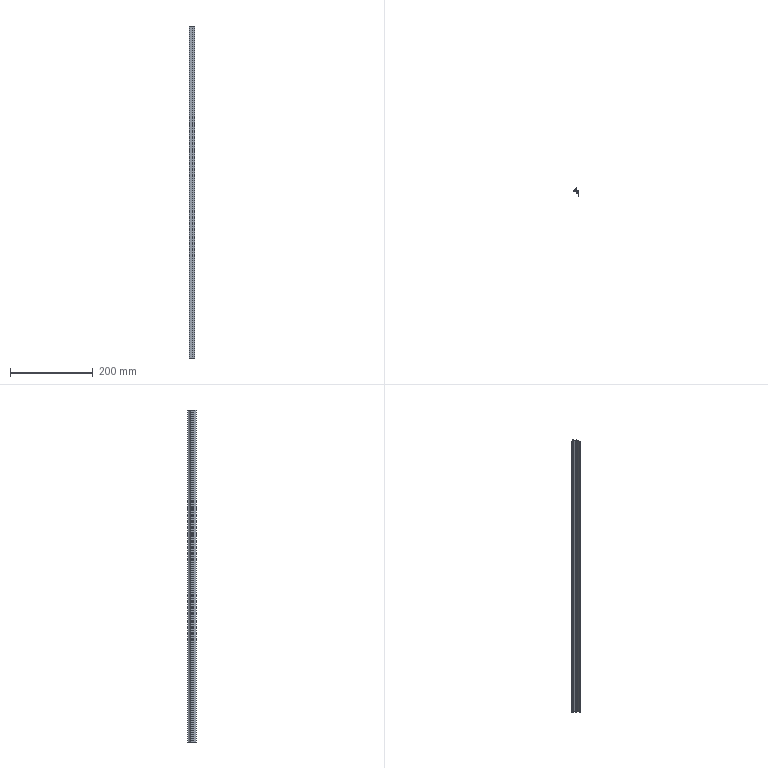Part | SolidWorks | features BaseBody 1, ICE 1, MoveFace 1 | 1 solid | 27 faces | box 14 x 20.3 x 800 mm | volume 40733 mm3 | plane 20 | cylinder 7 | commonest cylinder face diameters 0.387 x2 0.8 x2 0.4 x1 20 x1 22 x1
STEP:
#1=CARTESIAN_POINT('',(-5.304,-0.625,200.));
#2=VERTEX_POINT('',#1);
#3=CARTESIAN_POINT('',(-5.449,-0.8125,200.));
#4=VERTEX_POINT('',#3);
#5=CARTESIAN_POINT('',(-5.255,-0.8125,200.));
#6=DIRECTION('',(0.,0.,1.));
#7=DIRECTION('',(-1.,0.,0.));
#8=AXIS2_PLACEMENT_3D('',#5,#6,#7);
#9=CIRCLE('',#8,0.1937);
#10=EDGE_CURVE('',#2,#4,#9,.T.);
#11=ORIENTED_EDGE('',*,*,#10,.T.);
#12=CARTESIAN_POINT('',(-5.449,-0.8125,-600.));
#13=VERTEX_POINT('',#12);
#14=CARTESIAN_POINT('',(-5.449,-0.8125,230.));
#15=DIRECTION('',(0.,0.,-1.));
#16=VECTOR('',#15,1000.);
#17=LINE('',#14,#16);
#18=EDGE_CURVE('',#4,#13,#17,.T.);
#19=ORIENTED_EDGE('',*,*,#18,.T.);
#20=CARTESIAN_POINT('',(-5.304,-0.625,-600.));
#21=VERTEX_POINT('',#20);
#22=CARTESIAN_POINT('',(-5.255,-0.8125,-600.));
#23=DIRECTION('',(0.,0.,-1.));
#24=DIRECTION('',(1.,0.,0.));
#25=AXIS2_PLACEMENT_3D('',#22,#23,#24);
#26=CIRCLE('',#25,0.1937);
#27=EDGE_CURVE('',#13,#21,#26,.T.);
#28=ORIENTED_EDGE('',*,*,#27,.T.);
#29=CARTESIAN_POINT('',(-5.304,-0.625,230.));
#30=DIRECTION('',(0.,0.,-1.));
#31=VECTOR('',#30,1000.);
#32=LINE('',#29,#31);
#33=EDGE_CURVE('',#2,#21,#32,.T.);
#34=ORIENTED_EDGE('',*,*,#33,.F.);
#35=EDGE_LOOP('',(#11,#19,#28,#34));
#36=FACE_OUTER_BOUND('',#35,.T.);
#37=CARTESIAN_POINT('',(-5.255,-0.8125,230.));
#38=DIRECTION('',(0.,0.,-1.));
#39=DIRECTION('',(-1.,0.,0.));
#40=AXIS2_PLACEMENT_3D('',#37,#38,#39);
#41=CYLINDRICAL_SURFACE('',#40,0.1937);
#42=ADVANCED_FACE('',(#36),#41,.F.);
#43=CARTESIAN_POINT('',(5.,-1.,-600.));
#44=VERTEX_POINT('',#43);
#45=CARTESIAN_POINT('',(5.,-14.3,-600.));
#46=VERTEX_POINT('',#45);
#47=CARTESIAN_POINT('',(5.,29.623,-600.));
#48=DIRECTION('',(0.,-1.,0.));
#49=VECTOR('',#48,1000.);
#50=LINE('',#47,#49);
#51=EDGE_CURVE('',#44,#46,#50,.T.);
#52=ORIENTED_EDGE('',*,*,#51,.F.);
#53=CARTESIAN_POINT('',(5.,-1.,200.));
#54=VERTEX_POINT('',#53);
#55=CARTESIAN_POINT('',(5.,-1.,230.));
#56=DIRECTION('',(0.,0.,-1.));
#57=VECTOR('',#56,1000.);
#58=LINE('',#55,#57);
#59=EDGE_CURVE('',#54,#44,#58,.T.);
#60=ORIENTED_EDGE('',*,*,#59,.F.);
#61=CARTESIAN_POINT('',(5.,-14.3,200.));
#62=VERTEX_POINT('',#61);
#63=CARTESIAN_POINT('',(5.,-14.3,200.));
#64=DIRECTION('',(0.,1.,0.));
#65=VECTOR('',#64,1000.);
#66=LINE('',#63,#65);
#67=EDGE_CURVE('',#62,#54,#66,.T.);
#68=ORIENTED_EDGE('',*,*,#67,.F.);
#69=CARTESIAN_POINT('',(5.,-14.3,230.));
#70=DIRECTION('',(0.,0.,1.));
#71=VECTOR('',#70,1000.);
#72=LINE('',#69,#71);
#73=EDGE_CURVE('',#46,#62,#72,.T.);
#74=ORIENTED_EDGE('',*,*,#73,.F.);
#75=EDGE_LOOP('',(#52,#60,#68,#74));
#76=FACE_OUTER_BOUND('',#75,.T.);
#77=CARTESIAN_POINT('',(5.,-14.3,230.));
#78=DIRECTION('',(-1.,0.,0.));
#79=DIRECTION('',(0.,0.,1.));
#80=AXIS2_PLACEMENT_3D('',#77,#78,#79);
#81=PLANE('',#80);
#82=ADVANCED_FACE('',(#76),#81,.F.);
#83=CARTESIAN_POINT('',(-9.,-2.,-600.));
#84=VERTEX_POINT('',#83);
#85=CARTESIAN_POINT('',(-9.,-2.,200.));
#86=VERTEX_POINT('',#85);
#87=CARTESIAN_POINT('',(-9.,-2.,230.));
#88=DIRECTION('',(0.,0.,1.));
#89=VECTOR('',#88,1000.);
#90=LINE('',#87,#89);
#91=EDGE_CURVE('',#84,#86,#90,.T.);
#92=ORIENTED_EDGE('',*,*,#91,.F.);
#93=CARTESIAN_POINT('',(0.9,-2.,-600.));
#94=VERTEX_POINT('',#93);
#95=CARTESIAN_POINT('',(5.,-2.,-600.));
#96=DIRECTION('',(-1.,0.,0.));
#97=VECTOR('',#96,1000.);
#98=LINE('',#95,#97);
#99=EDGE_CURVE('',#94,#84,#98,.T.);
#100=ORIENTED_EDGE('',*,*,#99,.F.);
#101=CARTESIAN_POINT('',(0.9,-2.,200.));
#102=VERTEX_POINT('',#101);
#103=CARTESIAN_POINT('',(0.9,-2.,230.));
#104=DIRECTION('',(0.,0.,-1.));
#105=VECTOR('',#104,1000.);
#106=LINE('',#103,#105);
#107=EDGE_CURVE('',#102,#94,#106,.T.);
#108=ORIENTED_EDGE('',*,*,#107,.F.);
#109=CARTESIAN_POINT('',(5.,-2.,200.));
#110=DIRECTION('',(1.,0.,0.));
#111=VECTOR('',#110,1000.);
#112=LINE('',#109,#111);
#113=EDGE_CURVE('',#86,#102,#112,.T.);
#114=ORIENTED_EDGE('',*,*,#113,.F.);
#115=EDGE_LOOP('',(#92,#100,#108,#114));
#116=FACE_OUTER_BOUND('',#115,.T.);
#117=CARTESIAN_POINT('',(-9.,-2.,230.));
#118=DIRECTION('',(0.,1.,0.));
#119=DIRECTION('',(0.,0.,1.));
#120=AXIS2_PLACEMENT_3D('',#117,#118,#119);
#121=PLANE('',#120);
#122=ADVANCED_FACE('',(#116),#121,.F.);
#123=CARTESIAN_POINT('',(4.,-6.,200.));
#124=VERTEX_POINT('',#123);
#125=CARTESIAN_POINT('',(4.,-3.,200.));
#126=VERTEX_POINT('',#125);
#127=CARTESIAN_POINT('',(4.,29.623,200.));
#128=DIRECTION('',(0.,1.,0.));
#129=VECTOR('',#128,1000.);
#130=LINE('',#127,#129);
#131=EDGE_CURVE('',#124,#126,#130,.T.);
#132=ORIENTED_EDGE('',*,*,#131,.F.);
#133=CARTESIAN_POINT('',(1.,-6.,200.));
#134=VERTEX_POINT('',#133);
#135=CARTESIAN_POINT('',(5.,-6.,200.));
#136=DIRECTION('',(1.,0.,0.));
#137=VECTOR('',#136,1000.);
#138=LINE('',#135,#137);
#139=EDGE_CURVE('',#134,#124,#138,.T.);
#140=ORIENTED_EDGE('',*,*,#139,.F.);
#141=CARTESIAN_POINT('',(1.,-6.7,200.));
#142=VERTEX_POINT('',#141);
#143=CARTESIAN_POINT('',(1.,-6.,200.));
#144=DIRECTION('',(0.,-1.,0.));
#145=VECTOR('',#144,1000.);
#146=LINE('',#143,#145);
#147=EDGE_CURVE('',#134,#142,#146,.T.);
#148=ORIENTED_EDGE('',*,*,#147,.T.);
#149=CARTESIAN_POINT('',(-1.7,-6.7,200.));
#150=VERTEX_POINT('',#149);
#151=CARTESIAN_POINT('',(5.,-6.7,200.));
#152=DIRECTION('',(1.,0.,0.));
#153=VECTOR('',#152,1000.);
#154=LINE('',#151,#153);
#155=EDGE_CURVE('',#150,#142,#154,.T.);
#156=ORIENTED_EDGE('',*,*,#155,.F.);
#157=CARTESIAN_POINT('',(-1.7,-7.7,200.));
#158=VERTEX_POINT('',#157);
#159=CARTESIAN_POINT('',(-1.7,-6.7,200.));
#160=DIRECTION('',(0.,-1.,0.));
#161=VECTOR('',#160,1000.);
#162=LINE('',#159,#161);
#163=EDGE_CURVE('',#150,#158,#162,.T.);
#164=ORIENTED_EDGE('',*,*,#163,.T.);
#165=CARTESIAN_POINT('',(4.,-7.7,200.));
#166=VERTEX_POINT('',#165);
#167=CARTESIAN_POINT('',(5.,-7.7,200.));
#168=DIRECTION('',(-1.,0.,0.));
#169=VECTOR('',#168,1000.);
#170=LINE('',#167,#169);
#171=EDGE_CURVE('',#166,#158,#170,.T.);
#172=ORIENTED_EDGE('',*,*,#171,.F.);
#173=CARTESIAN_POINT('',(4.,-14.3,200.));
#174=VERTEX_POINT('',#173);
#175=CARTESIAN_POINT('',(4.,29.623,200.));
#176=DIRECTION('',(0.,1.,0.));
#177=VECTOR('',#176,1000.);
#178=LINE('',#175,#177);
#179=EDGE_CURVE('',#174,#166,#178,.T.);
#180=ORIENTED_EDGE('',*,*,#179,.F.);
#181=CARTESIAN_POINT('',(5.,-14.3,200.));
#182=DIRECTION('',(-1.,0.,0.));
#183=VECTOR('',#182,1000.);
#184=LINE('',#181,#183);
#185=EDGE_CURVE('',#62,#174,#184,.T.);
#186=ORIENTED_EDGE('',*,*,#185,.F.);
#187=ORIENTED_EDGE('',*,*,#67,.T.);
#188=CARTESIAN_POINT('',(-5.207,-1.,200.));
#189=VERTEX_POINT('',#188);
#190=CARTESIAN_POINT('',(5.,-1.,200.));
#191=DIRECTION('',(1.,0.,0.));
#192=VECTOR('',#191,1000.);
#193=LINE('',#190,#192);
#194=EDGE_CURVE('',#189,#54,#193,.T.);
#195=ORIENTED_EDGE('',*,*,#194,.F.);
#196=CARTESIAN_POINT('',(-5.255,-0.8125,200.));
#197=DIRECTION('',(0.,0.,1.));
#198=DIRECTION('',(-1.,0.,0.));
#199=AXIS2_PLACEMENT_3D('',#196,#197,#198);
#200=CIRCLE('',#199,0.1937);
#201=EDGE_CURVE('',#4,#189,#200,.T.);
#202=ORIENTED_EDGE('',*,*,#201,.F.);
#203=ORIENTED_EDGE('',*,*,#10,.F.);
#204=CARTESIAN_POINT('',(-1.368,3.063,200.));
#205=VERTEX_POINT('',#204);
#206=CARTESIAN_POINT('',(-10.628,9.,200.));
#207=DIRECTION('',(0.,0.,1.));
#208=DIRECTION('',(-1.,0.,0.));
#209=AXIS2_PLACEMENT_3D('',#206,#207,#208);
#210=CIRCLE('',#209,11.);
#211=EDGE_CURVE('',#2,#205,#210,.T.);
#212=ORIENTED_EDGE('',*,*,#211,.T.);
#213=CARTESIAN_POINT('',(-1.,2.955,200.));
#214=VERTEX_POINT('',#213);
#215=CARTESIAN_POINT('',(-1.2,2.955,200.));
#216=DIRECTION('',(0.,0.,1.));
#217=DIRECTION('',(-1.,0.,0.));
#218=AXIS2_PLACEMENT_3D('',#215,#216,#217);
#219=CIRCLE('',#218,0.2);
#220=EDGE_CURVE('',#214,#205,#219,.T.);
#221=ORIENTED_EDGE('',*,*,#220,.F.);
#222=CARTESIAN_POINT('',(-1.,1.5,200.));
#223=VERTEX_POINT('',#222);
#224=CARTESIAN_POINT('',(-1.,2.955,200.));
#225=DIRECTION('',(0.,1.,0.));
#226=VECTOR('',#225,1000.);
#227=LINE('',#224,#226);
#228=EDGE_CURVE('',#223,#214,#227,.T.);
#229=ORIENTED_EDGE('',*,*,#228,.F.);
#230=CARTESIAN_POINT('',(0.,1.5,200.));
#231=VERTEX_POINT('',#230);
#232=CARTESIAN_POINT('',(-1.,1.5,200.));
#233=DIRECTION('',(-1.,0.,0.));
#234=VECTOR('',#233,1000.);
#235=LINE('',#232,#234);
#236=EDGE_CURVE('',#231,#223,#235,.T.);
#237=ORIENTED_EDGE('',*,*,#236,.F.);
#238=CARTESIAN_POINT('',(0.,6.,200.));
#239=VERTEX_POINT('',#238);
#240=CARTESIAN_POINT('',(0.,1.5,200.));
#241=DIRECTION('',(0.,-1.,0.));
#242=VECTOR('',#241,1000.);
#243=LINE('',#240,#242);
#244=EDGE_CURVE('',#239,#231,#243,.T.);
#245=ORIENTED_EDGE('',*,*,#244,.F.);
#246=CARTESIAN_POINT('',(-0.8,6.,200.));
#247=VERTEX_POINT('',#246);
#248=CARTESIAN_POINT('',(0.,6.,200.));
#249=DIRECTION('',(1.,0.,0.));
#250=VECTOR('',#249,1000.);
#251=LINE('',#248,#250);
#252=EDGE_CURVE('',#247,#239,#251,.T.);
#253=ORIENTED_EDGE('',*,*,#252,.F.);
#254=CARTESIAN_POINT('',(-1.178,5.731,200.));
#255=VERTEX_POINT('',#254);
#256=CARTESIAN_POINT('',(-0.8,5.6,200.));
#257=DIRECTION('',(0.,0.,1.));
#258=DIRECTION('',(-1.,0.,0.));
#259=AXIS2_PLACEMENT_3D('',#256,#257,#258);
#260=CIRCLE('',#259,0.4);
#261=EDGE_CURVE('',#247,#255,#260,.T.);
#262=ORIENTED_EDGE('',*,*,#261,.T.);
#263=CARTESIAN_POINT('',(-8.678,-0.8077,200.));
#264=VERTEX_POINT('',#263);
#265=CARTESIAN_POINT('',(-10.628,9.,200.));
#266=DIRECTION('',(0.,0.,1.));
#267=DIRECTION('',(-1.,0.,0.));
#268=AXIS2_PLACEMENT_3D('',#265,#266,#267);
#269=CIRCLE('',#268,10.);
#270=EDGE_CURVE('',#264,#255,#269,.T.);
#271=ORIENTED_EDGE('',*,*,#270,.F.);
#272=CARTESIAN_POINT('',(-9.,-1.2,200.));
#273=VERTEX_POINT('',#272);
#274=CARTESIAN_POINT('',(-8.6,-1.2,200.));
#275=DIRECTION('',(0.,0.,1.));
#276=DIRECTION('',(-1.,0.,0.));
#277=AXIS2_PLACEMENT_3D('',#274,#275,#276);
#278=CIRCLE('',#277,0.4);
#279=EDGE_CURVE('',#264,#273,#278,.T.);
#280=ORIENTED_EDGE('',*,*,#279,.T.);
#281=CARTESIAN_POINT('',(-9.,8.,200.));
#282=DIRECTION('',(0.,-1.,0.));
#283=VECTOR('',#282,1000.);
#284=LINE('',#281,#283);
#285=EDGE_CURVE('',#273,#86,#284,.T.);
#286=ORIENTED_EDGE('',*,*,#285,.T.);
#287=ORIENTED_EDGE('',*,*,#113,.T.);
#288=CARTESIAN_POINT('',(0.9,-3.,200.));
#289=VERTEX_POINT('',#288);
#290=CARTESIAN_POINT('',(0.9,29.623,200.));
#291=DIRECTION('',(0.,1.,0.));
#292=VECTOR('',#291,1000.);
#293=LINE('',#290,#292);
#294=EDGE_CURVE('',#289,#102,#293,.T.);
#295=ORIENTED_EDGE('',*,*,#294,.F.);
#296=CARTESIAN_POINT('',(5.,-3.,200.));
#297=DIRECTION('',(-1.,0.,0.));
#298=VECTOR('',#297,1000.);
#299=LINE('',#296,#298);
#300=EDGE_CURVE('',#126,#289,#299,.T.);
#301=ORIENTED_EDGE('',*,*,#300,.F.);
#302=EDGE_LOOP('',(#132,#140,#148,#156,#164,#172,#180,#186,#187,#195,#202,#203,#212,#221,#229,#237,#245,#253,#262,#271,#280,#286,#287,#295,#301));
#303=FACE_OUTER_BOUND('',#302,.T.);
#304=CARTESIAN_POINT('',(5.,29.623,200.));
#305=DIRECTION('',(0.,0.,-1.));
#306=DIRECTION('',(-1.,0.,0.));
#307=AXIS2_PLACEMENT_3D('',#304,#305,#306);
#308=PLANE('',#307);
#309=ADVANCED_FACE('',(#303),#308,.F.);
#310=ORIENTED_EDGE('',*,*,#185,.T.);
#311=CARTESIAN_POINT('',(4.,-14.3,-600.));
#312=VERTEX_POINT('',#311);
#313=CARTESIAN_POINT('',(4.,-14.3,230.));
#314=DIRECTION('',(0.,0.,1.));
#315=VECTOR('',#314,1000.);
#316=LINE('',#313,#315);
#317=EDGE_CURVE('',#312,#174,#316,.T.);
#318=ORIENTED_EDGE('',*,*,#317,.F.);
#319=CARTESIAN_POINT('',(5.,-14.3,-600.));
#320=DIRECTION('',(-1.,0.,0.));
#321=VECTOR('',#320,1000.);
#322=LINE('',#319,#321);
#323=EDGE_CURVE('',#46,#312,#322,.T.);
#324=ORIENTED_EDGE('',*,*,#323,.F.);
#325=ORIENTED_EDGE('',*,*,#73,.T.);
#326=EDGE_LOOP('',(#310,#318,#324,#325));
#327=FACE_OUTER_BOUND('',#326,.T.);
#328=CARTESIAN_POINT('',(4.,-14.3,230.));
#329=DIRECTION('',(0.,1.,0.));
#330=DIRECTION('',(0.,0.,1.));
#331=AXIS2_PLACEMENT_3D('',#328,#329,#330);
#332=PLANE('',#331);
#333=ADVANCED_FACE('',(#327),#332,.F.);
#334=ORIENTED_EDGE('',*,*,#51,.T.);
#335=ORIENTED_EDGE('',*,*,#323,.T.);
#336=CARTESIAN_POINT('',(4.,-7.7,-600.));
#337=VERTEX_POINT('',#336);
#338=CARTESIAN_POINT('',(4.,-7.7,-600.));
#339=DIRECTION('',(0.,-1.,0.));
#340=VECTOR('',#339,1000.);
#341=LINE('',#338,#340);
#342=EDGE_CURVE('',#337,#312,#341,.T.);
#343=ORIENTED_EDGE('',*,*,#342,.F.);
#344=CARTESIAN_POINT('',(-1.7,-7.7,-600.));
#345=VERTEX_POINT('',#344);
#346=CARTESIAN_POINT('',(-1.7,-7.7,-600.));
#347=DIRECTION('',(1.,0.,0.));
#348=VECTOR('',#347,1000.);
#349=LINE('',#346,#348);
#350=EDGE_CURVE('',#345,#337,#349,.T.);
#351=ORIENTED_EDGE('',*,*,#350,.F.);
#352=CARTESIAN_POINT('',(-1.7,-6.7,-600.));
#353=VERTEX_POINT('',#352);
#354=CARTESIAN_POINT('',(-1.7,29.623,-600.));
#355=DIRECTION('',(0.,1.,0.));
#356=VECTOR('',#355,1000.);
#357=LINE('',#354,#356);
#358=EDGE_CURVE('',#345,#353,#357,.T.);
#359=ORIENTED_EDGE('',*,*,#358,.T.);
#360=CARTESIAN_POINT('',(1.,-6.7,-600.));
#361=VERTEX_POINT('',#360);
#362=CARTESIAN_POINT('',(1.,-6.7,-600.));
#363=DIRECTION('',(-1.,0.,0.));
#364=VECTOR('',#363,1000.);
#365=LINE('',#362,#364);
#366=EDGE_CURVE('',#361,#353,#365,.T.);
#367=ORIENTED_EDGE('',*,*,#366,.F.);
#368=CARTESIAN_POINT('',(1.,-6.,-600.));
#369=VERTEX_POINT('',#368);
#370=CARTESIAN_POINT('',(1.,29.623,-600.));
#371=DIRECTION('',(0.,1.,0.));
#372=VECTOR('',#371,1000.);
#373=LINE('',#370,#372);
#374=EDGE_CURVE('',#361,#369,#373,.T.);
#375=ORIENTED_EDGE('',*,*,#374,.T.);
#376=CARTESIAN_POINT('',(4.,-6.,-600.));
#377=VERTEX_POINT('',#376);
#378=CARTESIAN_POINT('',(4.,-6.,-600.));
#379=DIRECTION('',(-1.,0.,0.));
#380=VECTOR('',#379,1000.);
#381=LINE('',#378,#380);
#382=EDGE_CURVE('',#377,#369,#381,.T.);
#383=ORIENTED_EDGE('',*,*,#382,.F.);
#384=CARTESIAN_POINT('',(4.,-3.,-600.));
#385=VERTEX_POINT('',#384);
#386=CARTESIAN_POINT('',(4.,-3.,-600.));
#387=DIRECTION('',(0.,-1.,0.));
#388=VECTOR('',#387,1000.);
#389=LINE('',#386,#388);
#390=EDGE_CURVE('',#385,#377,#389,.T.);
#391=ORIENTED_EDGE('',*,*,#390,.F.);
#392=CARTESIAN_POINT('',(0.9,-3.,-600.));
#393=VERTEX_POINT('',#392);
#394=CARTESIAN_POINT('',(0.9,-3.,-600.));
#395=DIRECTION('',(1.,0.,0.));
#396=VECTOR('',#395,1000.);
#397=LINE('',#394,#396);
#398=EDGE_CURVE('',#393,#385,#397,.T.);
#399=ORIENTED_EDGE('',*,*,#398,.F.);
#400=CARTESIAN_POINT('',(0.9,-2.,-600.));
#401=DIRECTION('',(0.,-1.,0.));
#402=VECTOR('',#401,1000.);
#403=LINE('',#400,#402);
#404=EDGE_CURVE('',#94,#393,#403,.T.);
#405=ORIENTED_EDGE('',*,*,#404,.F.);
#406=ORIENTED_EDGE('',*,*,#99,.T.);
#407=CARTESIAN_POINT('',(-9.,-1.2,-600.));
#408=VERTEX_POINT('',#407);
#409=CARTESIAN_POINT('',(-9.,-1.2,-600.));
#410=DIRECTION('',(0.,-1.,0.));
#411=VECTOR('',#410,1000.);
#412=LINE('',#409,#411);
#413=EDGE_CURVE('',#408,#84,#412,.T.);
#414=ORIENTED_EDGE('',*,*,#413,.F.);
#415=CARTESIAN_POINT('',(-8.678,-0.8077,-600.));
#416=VERTEX_POINT('',#415);
#417=CARTESIAN_POINT('',(-8.6,-1.2,-600.));
#418=DIRECTION('',(0.,0.,-1.));
#419=DIRECTION('',(1.,0.,0.));
#420=AXIS2_PLACEMENT_3D('',#417,#418,#419);
#421=CIRCLE('',#420,0.4);
#422=EDGE_CURVE('',#408,#416,#421,.T.);
#423=ORIENTED_EDGE('',*,*,#422,.T.);
#424=CARTESIAN_POINT('',(-1.178,5.731,-600.));
#425=VERTEX_POINT('',#424);
#426=CARTESIAN_POINT('',(-10.628,9.,-600.));
#427=DIRECTION('',(0.,0.,-1.));
#428=DIRECTION('',(1.,0.,0.));
#429=AXIS2_PLACEMENT_3D('',#426,#427,#428);
#430=CIRCLE('',#429,10.);
#431=EDGE_CURVE('',#425,#416,#430,.T.);
#432=ORIENTED_EDGE('',*,*,#431,.F.);
#433=CARTESIAN_POINT('',(-0.8,6.,-600.));
#434=VERTEX_POINT('',#433);
#435=CARTESIAN_POINT('',(-0.8,5.6,-600.));
#436=DIRECTION('',(0.,0.,-1.));
#437=DIRECTION('',(1.,0.,0.));
#438=AXIS2_PLACEMENT_3D('',#435,#436,#437);
#439=CIRCLE('',#438,0.4);
#440=EDGE_CURVE('',#425,#434,#439,.T.);
#441=ORIENTED_EDGE('',*,*,#440,.T.);
#442=CARTESIAN_POINT('',(0.,6.,-600.));
#443=VERTEX_POINT('',#442);
#444=CARTESIAN_POINT('',(0.,6.,-600.));
#445=DIRECTION('',(-1.,0.,0.));
#446=VECTOR('',#445,1000.);
#447=LINE('',#444,#446);
#448=EDGE_CURVE('',#443,#434,#447,.T.);
#449=ORIENTED_EDGE('',*,*,#448,.F.);
#450=CARTESIAN_POINT('',(0.,1.5,-600.));
#451=VERTEX_POINT('',#450);
#452=CARTESIAN_POINT('',(0.,1.5,-600.));
#453=DIRECTION('',(0.,1.,0.));
#454=VECTOR('',#453,1000.);
#455=LINE('',#452,#454);
#456=EDGE_CURVE('',#451,#443,#455,.T.);
#457=ORIENTED_EDGE('',*,*,#456,.F.);
#458=CARTESIAN_POINT('',(-1.,1.5,-600.));
#459=VERTEX_POINT('',#458);
#460=CARTESIAN_POINT('',(-1.,1.5,-600.));
#461=DIRECTION('',(1.,0.,0.));
#462=VECTOR('',#461,1000.);
#463=LINE('',#460,#462);
#464=EDGE_CURVE('',#459,#451,#463,.T.);
#465=ORIENTED_EDGE('',*,*,#464,.F.);
#466=CARTESIAN_POINT('',(-1.,2.955,-600.));
#467=VERTEX_POINT('',#466);
#468=CARTESIAN_POINT('',(-1.,2.955,-600.));
#469=DIRECTION('',(0.,-1.,0.));
#470=VECTOR('',#469,1000.);
#471=LINE('',#468,#470);
#472=EDGE_CURVE('',#467,#459,#471,.T.);
#473=ORIENTED_EDGE('',*,*,#472,.F.);
#474=CARTESIAN_POINT('',(-1.368,3.063,-600.));
#475=VERTEX_POINT('',#474);
#476=CARTESIAN_POINT('',(-1.2,2.955,-600.));
#477=DIRECTION('',(0.,0.,-1.));
#478=DIRECTION('',(1.,0.,0.));
#479=AXIS2_PLACEMENT_3D('',#476,#477,#478);
#480=CIRCLE('',#479,0.2);
#481=EDGE_CURVE('',#475,#467,#480,.T.);
#482=ORIENTED_EDGE('',*,*,#481,.F.);
#483=CARTESIAN_POINT('',(-10.628,9.,-600.));
#484=DIRECTION('',(0.,0.,-1.));
#485=DIRECTION('',(1.,0.,0.));
#486=AXIS2_PLACEMENT_3D('',#483,#484,#485);
#487=CIRCLE('',#486,11.);
#488=EDGE_CURVE('',#475,#21,#487,.T.);
#489=ORIENTED_EDGE('',*,*,#488,.T.);
#490=ORIENTED_EDGE('',*,*,#27,.F.);
#491=CARTESIAN_POINT('',(-5.207,-1.,-600.));
#492=VERTEX_POINT('',#491);
#493=CARTESIAN_POINT('',(-5.255,-0.8125,-600.));
#494=DIRECTION('',(0.,0.,-1.));
#495=DIRECTION('',(1.,0.,0.));
#496=AXIS2_PLACEMENT_3D('',#493,#494,#495);
#497=CIRCLE('',#496,0.1937);
#498=EDGE_CURVE('',#492,#13,#497,.T.);
#499=ORIENTED_EDGE('',*,*,#498,.F.);
#500=CARTESIAN_POINT('',(5.,-1.,-600.));
#501=DIRECTION('',(-1.,0.,0.));
#502=VECTOR('',#501,1000.);
#503=LINE('',#500,#502);
#504=EDGE_CURVE('',#44,#492,#503,.T.);
#505=ORIENTED_EDGE('',*,*,#504,.F.);
#506=EDGE_LOOP('',(#334,#335,#343,#351,#359,#367,#375,#383,#391,#399,#405,#406,#414,#423,#432,#441,#449,#457,#465,#473,#482,#489,#490,#499,#505));
#507=FACE_OUTER_BOUND('',#506,.T.);
#508=CARTESIAN_POINT('',(5.,29.623,-600.));
#509=DIRECTION('',(0.,0.,1.));
#510=DIRECTION('',(1.,0.,0.));
#511=AXIS2_PLACEMENT_3D('',#508,#509,#510);
#512=PLANE('',#511);
#513=ADVANCED_FACE('',(#507),#512,.F.);
#514=ORIENTED_EDGE('',*,*,#59,.T.);
#515=ORIENTED_EDGE('',*,*,#504,.T.);
#516=CARTESIAN_POINT('',(-5.207,-1.,230.));
#517=DIRECTION('',(0.,0.,-1.));
#518=VECTOR('',#517,1000.);
#519=LINE('',#516,#518);
#520=EDGE_CURVE('',#189,#492,#519,.T.);
#521=ORIENTED_EDGE('',*,*,#520,.F.);
#522=ORIENTED_EDGE('',*,*,#194,.T.);
#523=EDGE_LOOP('',(#514,#515,#521,#522));
#524=FACE_OUTER_BOUND('',#523,.T.);
#525=CARTESIAN_POINT('',(5.,-1.,230.));
#526=DIRECTION('',(0.,-1.,0.));
#527=DIRECTION('',(0.,0.,-1.));
#528=AXIS2_PLACEMENT_3D('',#525,#526,#527);
#529=PLANE('',#528);
#530=ADVANCED_FACE('',(#524),#529,.F.);
#531=CARTESIAN_POINT('',(-9.,-1.2,230.));
#532=DIRECTION('',(0.,0.,1.));
#533=VECTOR('',#532,1000.);
#534=LINE('',#531,#533);
#535=EDGE_CURVE('',#408,#273,#534,.T.);
#536=ORIENTED_EDGE('',*,*,#535,.F.);
#537=ORIENTED_EDGE('',*,*,#413,.T.);
#538=ORIENTED_EDGE('',*,*,#91,.T.);
#539=ORIENTED_EDGE('',*,*,#285,.F.);
#540=EDGE_LOOP('',(#536,#537,#538,#539));
#541=FACE_OUTER_BOUND('',#540,.T.);
#542=CARTESIAN_POINT('',(-9.,-1.2,230.));
#543=DIRECTION('',(1.,0.,0.));
#544=DIRECTION('',(0.,0.,-1.));
#545=AXIS2_PLACEMENT_3D('',#542,#543,#544);
#546=PLANE('',#545);
#547=ADVANCED_FACE('',(#541),#546,.F.);
#548=ORIENTED_EDGE('',*,*,#294,.T.);
#549=ORIENTED_EDGE('',*,*,#107,.T.);
#550=ORIENTED_EDGE('',*,*,#404,.T.);
#551=CARTESIAN_POINT('',(0.9,-3.,230.));
#552=DIRECTION('',(0.,0.,-1.));
#553=VECTOR('',#552,1000.);
#554=LINE('',#551,#553);
#555=EDGE_CURVE('',#289,#393,#554,.T.);
#556=ORIENTED_EDGE('',*,*,#555,.F.);
#557=EDGE_LOOP('',(#548,#549,#550,#556));
#558=FACE_OUTER_BOUND('',#557,.T.);
#559=CARTESIAN_POINT('',(0.9,-2.,230.));
#560=DIRECTION('',(1.,0.,0.));
#561=DIRECTION('',(0.,0.,-1.));
#562=AXIS2_PLACEMENT_3D('',#559,#560,#561);
#563=PLANE('',#562);
#564=ADVANCED_FACE('',(#558),#563,.F.);
#565=ORIENTED_EDGE('',*,*,#300,.T.);
#566=ORIENTED_EDGE('',*,*,#555,.T.);
#567=ORIENTED_EDGE('',*,*,#398,.T.);
#568=CARTESIAN_POINT('',(4.,-3.,230.));
#569=DIRECTION('',(0.,0.,-1.));
#570=VECTOR('',#569,1000.);
#571=LINE('',#568,#570);
#572=EDGE_CURVE('',#126,#385,#571,.T.);
#573=ORIENTED_EDGE('',*,*,#572,.F.);
#574=EDGE_LOOP('',(#565,#566,#567,#573));
#575=FACE_OUTER_BOUND('',#574,.T.);
#576=CARTESIAN_POINT('',(0.9,-3.,230.));
#577=DIRECTION('',(0.,1.,0.));
#578=DIRECTION('',(0.,0.,1.));
#579=AXIS2_PLACEMENT_3D('',#576,#577,#578);
#580=PLANE('',#579);
#581=ADVANCED_FACE('',(#575),#580,.F.);
#582=ORIENTED_EDGE('',*,*,#131,.T.);
#583=ORIENTED_EDGE('',*,*,#572,.T.);
#584=ORIENTED_EDGE('',*,*,#390,.T.);
#585=CARTESIAN_POINT('',(4.,-6.,230.));
#586=DIRECTION('',(0.,0.,-1.));
#587=VECTOR('',#586,1000.);
#588=LINE('',#585,#587);
#589=EDGE_CURVE('',#124,#377,#588,.T.);
#590=ORIENTED_EDGE('',*,*,#589,.F.);
#591=EDGE_LOOP('',(#582,#583,#584,#590));
#592=FACE_OUTER_BOUND('',#591,.T.);
#593=CARTESIAN_POINT('',(4.,-3.,230.));
#594=DIRECTION('',(1.,0.,0.));
#595=DIRECTION('',(0.,0.,-1.));
#596=AXIS2_PLACEMENT_3D('',#593,#594,#595);
#597=PLANE('',#596);
#598=ADVANCED_FACE('',(#592),#597,.F.);
#599=ORIENTED_EDGE('',*,*,#139,.T.);
#600=ORIENTED_EDGE('',*,*,#589,.T.);
#601=ORIENTED_EDGE('',*,*,#382,.T.);
#602=CARTESIAN_POINT('',(1.,-6.,230.));
#603=DIRECTION('',(0.,0.,-1.));
#604=VECTOR('',#603,1000.);
#605=LINE('',#602,#604);
#606=EDGE_CURVE('',#134,#369,#605,.T.);
#607=ORIENTED_EDGE('',*,*,#606,.F.);
#608=EDGE_LOOP('',(#599,#600,#601,#607));
#609=FACE_OUTER_BOUND('',#608,.T.);
#610=CARTESIAN_POINT('',(4.,-6.,230.));
#611=DIRECTION('',(0.,-1.,0.));
#612=DIRECTION('',(0.,0.,-1.));
#613=AXIS2_PLACEMENT_3D('',#610,#611,#612);
#614=PLANE('',#613);
#615=ADVANCED_FACE('',(#609),#614,.F.);
#616=ORIENTED_EDGE('',*,*,#155,.T.);
#617=CARTESIAN_POINT('',(1.,-6.7,230.));
#618=DIRECTION('',(0.,0.,1.));
#619=VECTOR('',#618,1000.);
#620=LINE('',#617,#619);
#621=EDGE_CURVE('',#361,#142,#620,.T.);
#622=ORIENTED_EDGE('',*,*,#621,.F.);
#623=ORIENTED_EDGE('',*,*,#366,.T.);
#624=CARTESIAN_POINT('',(-1.7,-6.7,230.));
#625=DIRECTION('',(0.,0.,-1.));
#626=VECTOR('',#625,1000.);
#627=LINE('',#624,#626);
#628=EDGE_CURVE('',#150,#353,#627,.T.);
#629=ORIENTED_EDGE('',*,*,#628,.F.);
#630=EDGE_LOOP('',(#616,#622,#623,#629));
#631=FACE_OUTER_BOUND('',#630,.T.);
#632=CARTESIAN_POINT('',(1.,-6.7,230.));
#633=DIRECTION('',(0.,-1.,0.));
#634=DIRECTION('',(0.,0.,-1.));
#635=AXIS2_PLACEMENT_3D('',#632,#633,#634);
#636=PLANE('',#635);
#637=ADVANCED_FACE('',(#631),#636,.F.);
#638=ORIENTED_EDGE('',*,*,#171,.T.);
#639=CARTESIAN_POINT('',(-1.7,-7.7,230.));
#640=DIRECTION('',(0.,0.,1.));
#641=VECTOR('',#640,1000.);
#642=LINE('',#639,#641);
#643=EDGE_CURVE('',#345,#158,#642,.T.);
#644=ORIENTED_EDGE('',*,*,#643,.F.);
#645=ORIENTED_EDGE('',*,*,#350,.T.);
#646=CARTESIAN_POINT('',(4.,-7.7,230.));
#647=DIRECTION('',(0.,0.,-1.));
#648=VECTOR('',#647,1000.);
#649=LINE('',#646,#648);
#650=EDGE_CURVE('',#166,#337,#649,.T.);
#651=ORIENTED_EDGE('',*,*,#650,.F.);
#652=EDGE_LOOP('',(#638,#644,#645,#651));
#653=FACE_OUTER_BOUND('',#652,.T.);
#654=CARTESIAN_POINT('',(-1.7,-7.7,230.));
#655=DIRECTION('',(0.,1.,0.));
#656=DIRECTION('',(0.,0.,1.));
#657=AXIS2_PLACEMENT_3D('',#654,#655,#656);
#658=PLANE('',#657);
#659=ADVANCED_FACE('',(#653),#658,.F.);
#660=ORIENTED_EDGE('',*,*,#179,.T.);
#661=ORIENTED_EDGE('',*,*,#650,.T.);
#662=ORIENTED_EDGE('',*,*,#342,.T.);
#663=ORIENTED_EDGE('',*,*,#317,.T.);
#664=EDGE_LOOP('',(#660,#661,#662,#663));
#665=FACE_OUTER_BOUND('',#664,.T.);
#666=CARTESIAN_POINT('',(4.,-7.7,230.));
#667=DIRECTION('',(1.,0.,0.));
#668=DIRECTION('',(0.,0.,-1.));
#669=AXIS2_PLACEMENT_3D('',#666,#667,#668);
#670=PLANE('',#669);
#671=ADVANCED_FACE('',(#665),#670,.F.);
#672=ORIENTED_EDGE('',*,*,#18,.F.);
#673=ORIENTED_EDGE('',*,*,#201,.T.);
#674=ORIENTED_EDGE('',*,*,#520,.T.);
#675=ORIENTED_EDGE('',*,*,#498,.T.);
#676=EDGE_LOOP('',(#672,#673,#674,#675));
#677=FACE_OUTER_BOUND('',#676,.T.);
#678=CARTESIAN_POINT('',(-5.255,-0.8125,230.));
#679=DIRECTION('',(0.,0.,-1.));
#680=DIRECTION('',(-1.,0.,0.));
#681=AXIS2_PLACEMENT_3D('',#678,#679,#680);
#682=CYLINDRICAL_SURFACE('',#681,0.1937);
#683=ADVANCED_FACE('',(#677),#682,.F.);
#684=CARTESIAN_POINT('',(-1.,2.955,230.));
#685=DIRECTION('',(0.,0.,1.));
#686=VECTOR('',#685,1000.);
#687=LINE('',#684,#686);
#688=EDGE_CURVE('',#467,#214,#687,.T.);
#689=ORIENTED_EDGE('',*,*,#688,.F.);
#690=ORIENTED_EDGE('',*,*,#472,.T.);
#691=CARTESIAN_POINT('',(-1.,1.5,230.));
#692=DIRECTION('',(0.,0.,-1.));
#693=VECTOR('',#692,1000.);
#694=LINE('',#691,#693);
#695=EDGE_CURVE('',#223,#459,#694,.T.);
#696=ORIENTED_EDGE('',*,*,#695,.F.);
#697=ORIENTED_EDGE('',*,*,#228,.T.);
#698=EDGE_LOOP('',(#689,#690,#696,#697));
#699=FACE_OUTER_BOUND('',#698,.T.);
#700=CARTESIAN_POINT('',(-1.,2.955,230.));
#701=DIRECTION('',(1.,0.,0.));
#702=DIRECTION('',(0.,0.,-1.));
#703=AXIS2_PLACEMENT_3D('',#700,#701,#702);
#704=PLANE('',#703);
#705=ADVANCED_FACE('',(#699),#704,.F.);
#706=ORIENTED_EDGE('',*,*,#488,.F.);
#707=CARTESIAN_POINT('',(-1.368,3.063,230.));
#708=DIRECTION('',(0.,0.,1.));
#709=VECTOR('',#708,1000.);
#710=LINE('',#707,#709);
#711=EDGE_CURVE('',#475,#205,#710,.T.);
#712=ORIENTED_EDGE('',*,*,#711,.T.);
#713=ORIENTED_EDGE('',*,*,#211,.F.);
#714=ORIENTED_EDGE('',*,*,#33,.T.);
#715=EDGE_LOOP('',(#706,#712,#713,#714));
#716=FACE_OUTER_BOUND('',#715,.T.);
#717=CARTESIAN_POINT('',(-10.628,9.,230.));
#718=DIRECTION('',(0.,0.,-1.));
#719=DIRECTION('',(-1.,0.,0.));
#720=AXIS2_PLACEMENT_3D('',#717,#718,#719);
#721=CYLINDRICAL_SURFACE('',#720,11.);
#722=ADVANCED_FACE('',(#716),#721,.T.);
#723=CARTESIAN_POINT('',(-1.178,5.731,230.));
#724=DIRECTION('',(0.,0.,1.));
#725=VECTOR('',#724,1000.);
#726=LINE('',#723,#725);
#727=EDGE_CURVE('',#425,#255,#726,.T.);
#728=ORIENTED_EDGE('',*,*,#727,.F.);
#729=ORIENTED_EDGE('',*,*,#431,.T.);
#730=CARTESIAN_POINT('',(-8.678,-0.8077,230.));
#731=DIRECTION('',(0.,0.,-1.));
#732=VECTOR('',#731,1000.);
#733=LINE('',#730,#732);
#734=EDGE_CURVE('',#264,#416,#733,.T.);
#735=ORIENTED_EDGE('',*,*,#734,.F.);
#736=ORIENTED_EDGE('',*,*,#270,.T.);
#737=EDGE_LOOP('',(#728,#729,#735,#736));
#738=FACE_OUTER_BOUND('',#737,.T.);
#739=CARTESIAN_POINT('',(-10.628,9.,230.));
#740=DIRECTION('',(0.,0.,-1.));
#741=DIRECTION('',(-1.,0.,0.));
#742=AXIS2_PLACEMENT_3D('',#739,#740,#741);
#743=CYLINDRICAL_SURFACE('',#742,10.);
#744=ADVANCED_FACE('',(#738),#743,.F.);
#745=CARTESIAN_POINT('',(0.,1.5,230.));
#746=DIRECTION('',(0.,0.,1.));
#747=VECTOR('',#746,1000.);
#748=LINE('',#745,#747);
#749=EDGE_CURVE('',#451,#231,#748,.T.);
#750=ORIENTED_EDGE('',*,*,#749,.F.);
#751=ORIENTED_EDGE('',*,*,#456,.T.);
#752=CARTESIAN_POINT('',(0.,6.,230.));
#753=DIRECTION('',(0.,0.,-1.));
#754=VECTOR('',#753,1000.);
#755=LINE('',#752,#754);
#756=EDGE_CURVE('',#239,#443,#755,.T.);
#757=ORIENTED_EDGE('',*,*,#756,.F.);
#758=ORIENTED_EDGE('',*,*,#244,.T.);
#759=EDGE_LOOP('',(#750,#751,#757,#758));
#760=FACE_OUTER_BOUND('',#759,.T.);
#761=CARTESIAN_POINT('',(0.,1.5,230.));
#762=DIRECTION('',(-1.,0.,0.));
#763=DIRECTION('',(0.,0.,1.));
#764=AXIS2_PLACEMENT_3D('',#761,#762,#763);
#765=PLANE('',#764);
#766=ADVANCED_FACE('',(#760),#765,.F.);
#767=ORIENTED_EDGE('',*,*,#422,.F.);
#768=ORIENTED_EDGE('',*,*,#535,.T.);
#769=ORIENTED_EDGE('',*,*,#279,.F.);
#770=ORIENTED_EDGE('',*,*,#734,.T.);
#771=EDGE_LOOP('',(#767,#768,#769,#770));
#772=FACE_OUTER_BOUND('',#771,.T.);
#773=CARTESIAN_POINT('',(-8.6,-1.2,230.));
#774=DIRECTION('',(0.,0.,-1.));
#775=DIRECTION('',(-1.,0.,0.));
#776=AXIS2_PLACEMENT_3D('',#773,#774,#775);
#777=CYLINDRICAL_SURFACE('',#776,0.4);
#778=ADVANCED_FACE('',(#772),#777,.T.);
#779=ORIENTED_EDGE('',*,*,#147,.F.);
#780=ORIENTED_EDGE('',*,*,#606,.T.);
#781=ORIENTED_EDGE('',*,*,#374,.F.);
#782=ORIENTED_EDGE('',*,*,#621,.T.);
#783=EDGE_LOOP('',(#779,#780,#781,#782));
#784=FACE_OUTER_BOUND('',#783,.T.);
#785=CARTESIAN_POINT('',(1.,-6.,230.));
#786=DIRECTION('',(1.,0.,0.));
#787=DIRECTION('',(0.,0.,-1.));
#788=AXIS2_PLACEMENT_3D('',#785,#786,#787);
#789=PLANE('',#788);
#790=ADVANCED_FACE('',(#784),#789,.F.);
#791=ORIENTED_EDGE('',*,*,#163,.F.);
#792=ORIENTED_EDGE('',*,*,#628,.T.);
#793=ORIENTED_EDGE('',*,*,#358,.F.);
#794=ORIENTED_EDGE('',*,*,#643,.T.);
#795=EDGE_LOOP('',(#791,#792,#793,#794));
#796=FACE_OUTER_BOUND('',#795,.T.);
#797=CARTESIAN_POINT('',(-1.7,-6.7,230.));
#798=DIRECTION('',(1.,0.,0.));
#799=DIRECTION('',(0.,0.,-1.));
#800=AXIS2_PLACEMENT_3D('',#797,#798,#799);
#801=PLANE('',#800);
#802=ADVANCED_FACE('',(#796),#801,.F.);
#803=ORIENTED_EDGE('',*,*,#711,.F.);
#804=ORIENTED_EDGE('',*,*,#481,.T.);
#805=ORIENTED_EDGE('',*,*,#688,.T.);
#806=ORIENTED_EDGE('',*,*,#220,.T.);
#807=EDGE_LOOP('',(#803,#804,#805,#806));
#808=FACE_OUTER_BOUND('',#807,.T.);
#809=CARTESIAN_POINT('',(-1.2,2.955,230.));
#810=DIRECTION('',(0.,0.,-1.));
#811=DIRECTION('',(-1.,0.,0.));
#812=AXIS2_PLACEMENT_3D('',#809,#810,#811);
#813=CYLINDRICAL_SURFACE('',#812,0.2);
#814=ADVANCED_FACE('',(#808),#813,.F.);
#815=ORIENTED_EDGE('',*,*,#695,.T.);
#816=ORIENTED_EDGE('',*,*,#464,.T.);
#817=ORIENTED_EDGE('',*,*,#749,.T.);
#818=ORIENTED_EDGE('',*,*,#236,.T.);
#819=EDGE_LOOP('',(#815,#816,#817,#818));
#820=FACE_OUTER_BOUND('',#819,.T.);
#821=CARTESIAN_POINT('',(-1.,1.5,230.));
#822=DIRECTION('',(0.,1.,0.));
#823=DIRECTION('',(0.,0.,1.));
#824=AXIS2_PLACEMENT_3D('',#821,#822,#823);
#825=PLANE('',#824);
#826=ADVANCED_FACE('',(#820),#825,.F.);
#827=ORIENTED_EDGE('',*,*,#440,.F.);
#828=ORIENTED_EDGE('',*,*,#727,.T.);
#829=ORIENTED_EDGE('',*,*,#261,.F.);
#830=CARTESIAN_POINT('',(-0.8,6.,230.));
#831=DIRECTION('',(0.,0.,-1.));
#832=VECTOR('',#831,1000.);
#833=LINE('',#830,#832);
#834=EDGE_CURVE('',#247,#434,#833,.T.);
#835=ORIENTED_EDGE('',*,*,#834,.T.);
#836=EDGE_LOOP('',(#827,#828,#829,#835));
#837=FACE_OUTER_BOUND('',#836,.T.);
#838=CARTESIAN_POINT('',(-0.8,5.6,230.));
#839=DIRECTION('',(0.,0.,-1.));
#840=DIRECTION('',(-1.,0.,0.));
#841=AXIS2_PLACEMENT_3D('',#838,#839,#840);
#842=CYLINDRICAL_SURFACE('',#841,0.4);
#843=ADVANCED_FACE('',(#837),#842,.T.);
#844=ORIENTED_EDGE('',*,*,#756,.T.);
#845=ORIENTED_EDGE('',*,*,#448,.T.);
#846=ORIENTED_EDGE('',*,*,#834,.F.);
#847=ORIENTED_EDGE('',*,*,#252,.T.);
#848=EDGE_LOOP('',(#844,#845,#846,#847));
#849=FACE_OUTER_BOUND('',#848,.T.);
#850=CARTESIAN_POINT('',(0.,6.,230.));
#851=DIRECTION('',(0.,-1.,0.));
#852=DIRECTION('',(0.,0.,-1.));
#853=AXIS2_PLACEMENT_3D('',#850,#851,#852);
#854=PLANE('',#853);
#855=ADVANCED_FACE('',(#849),#854,.F.);
#856=CLOSED_SHELL('',(#42,#82,#122,#309,#333,#513,#530,#547,#564,#581,#598,#615,#637,#659,#671,#683,#705,#722,#744,#766,#778,#790,#802,#814,#826,#843,#855));
#857=MANIFOLD_SOLID_BREP('',#856);
#858=CARTESIAN_POINT('',(0.,0.,0.));
#859=DIRECTION('',(0.,0.,1.));
#860=DIRECTION('',(1.,0.,0.));
#861=AXIS2_PLACEMENT_3D('',#858,#859,#860);
#862=(LENGTH_UNIT()NAMED_UNIT(*)SI_UNIT(.MILLI.,.METRE.));
#863=UNCERTAINTY_MEASURE_WITH_UNIT(LENGTH_MEASURE(0.00001),#862,'','');
#864=(NAMED_UNIT(*)PLANE_ANGLE_UNIT()SI_UNIT($,.RADIAN.));
#865=(NAMED_UNIT(*)SI_UNIT($,.STERADIAN.)SOLID_ANGLE_UNIT());
#866=(GEOMETRIC_REPRESENTATION_CONTEXT(3)GLOBAL_UNCERTAINTY_ASSIGNED_CONTEXT((#863))GLOBAL_UNIT_ASSIGNED_CONTEXT((#862,#864,#865))REPRESENTATION_CONTEXT('',''));
#867=ADVANCED_BREP_SHAPE_REPRESENTATION('',(#857,#861),#866);